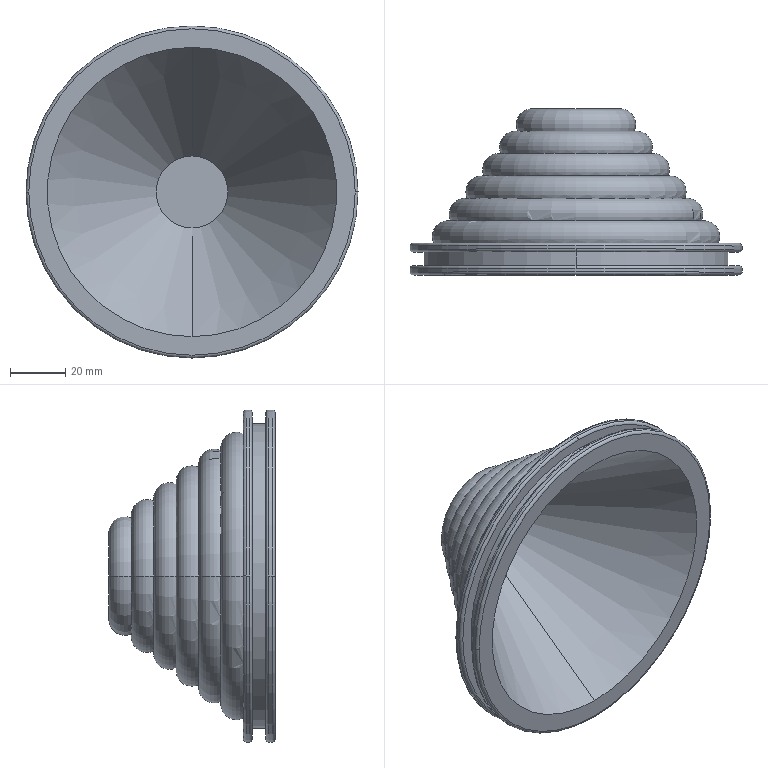Part | STEP file | Tower-type sealing ring | 1 solid | 34 faces | box 120 x 60.067 x 120 mm | volume 130972 mm3 | torus 20 | cylinder 6 | plane 6 | cone 2 | commonest cylinder face diameters 120 x4 110 x2